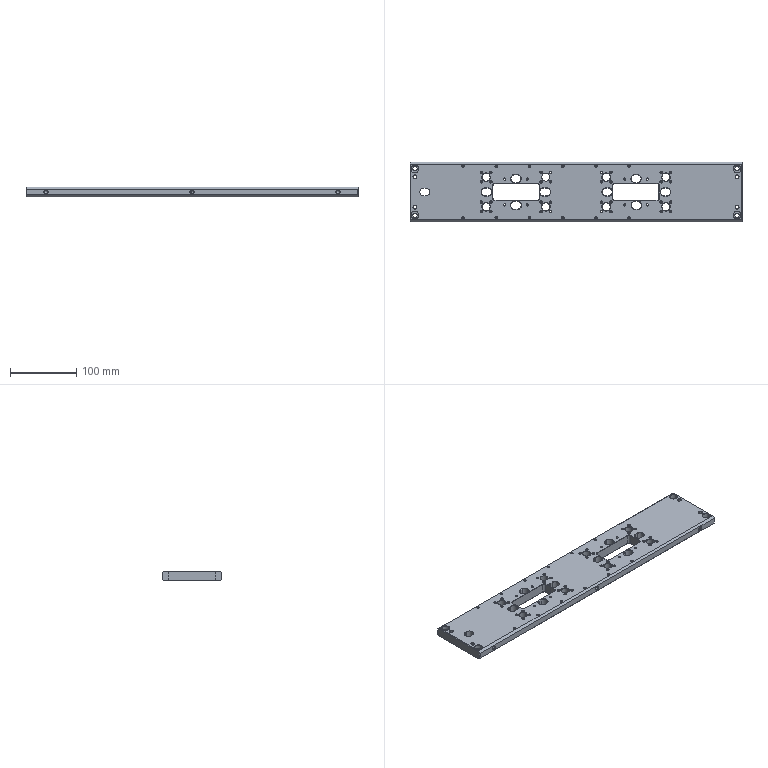Part | SolidWorks | features HoleWzd 8, Chamfer 5, Cut 4, LPattern 3, Extrusion 1, Fillet 1, MirrorPattern 1 | 1 solid | 631 faces | box 500 x 90 x 15 mm | volume 566353 mm3 | cone 330 | cylinder 201 | plane 100 | commonest cylinder face diameters 2.5 x88 12 x45 5 x20 3.3 x16 11 x16 6 x8